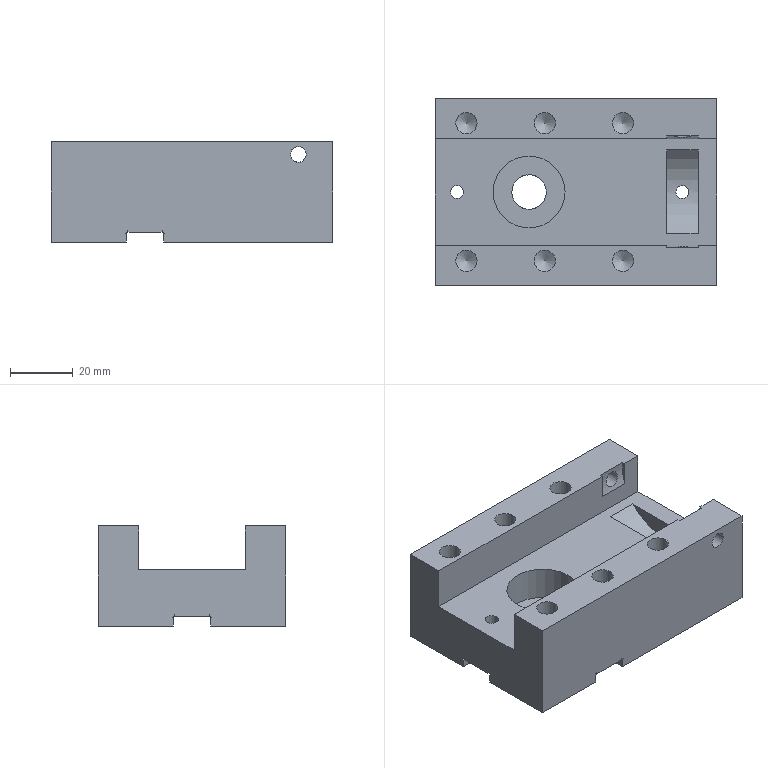Part | NX | features DATUM_CSYS 20, SKETCH 19, HOLE PACKAGE 9, SIMPLE HOLE 9, SYMBOLIC_THREAD 9, EXTRACT_FACE 8, EXTRUDE 7, Instance Feature 6, BLOCK 2, CYLINDER 2, Pattern Feature 2, BLEND 1, CPROJ 1 | 3 solids | 99 faces | box 90 x 60 x 32 mm | volume 114243 mm3 | plane 66 | cylinder 27 | cone 6 | commonest cylinder face diameters 1 x8 6.8 x6 11 x3 36 x3 1.008 x2 4.2 x2